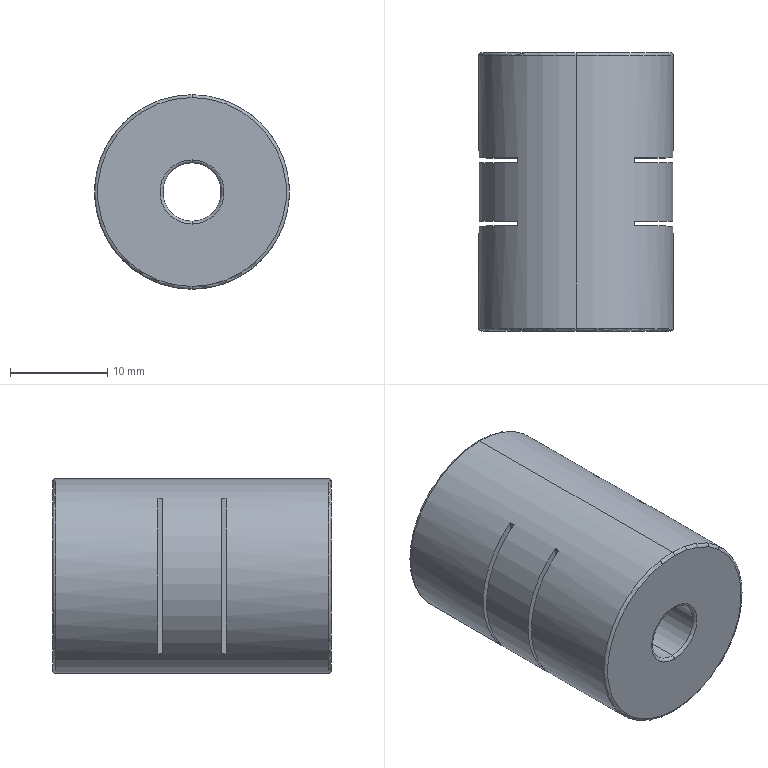Part | STEP file | GCPSW20-6-6 | 1 solid | 34 faces | box 20 x 28.6 x 20 mm | volume 8036 mm3 | plane 14 | torus 8 | cylinder 8 | cone 4 | commonest cylinder face diameters 2.5 x4 6 x2 20 x2